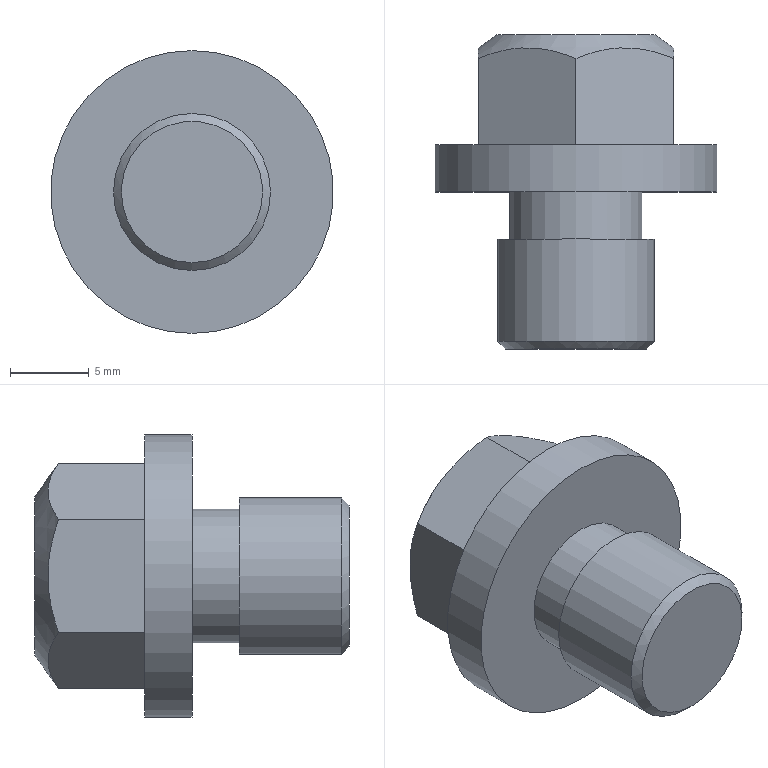Part | NX | 1 solid | 16 faces | box 18 x 20 x 18 mm | volume 2389 mm3 | plane 11 | cylinder 3 | cone 2 | commonest cylinder face diameters 8.5 x1 10 x1 18 x1
STEP:
#1=CARTESIAN_POINT('',(-6.227,18.49,-3.595));
#2=VERTEX_POINT('',#1);
#3=CARTESIAN_POINT('',(-6.227,18.49,3.595));
#4=VERTEX_POINT('',#3);
#5=CARTESIAN_POINT('',(-6.227,18.49,-3.595));
#6=CARTESIAN_POINT('',(-6.227,18.901,-2.433));
#7=CARTESIAN_POINT('',(-6.227,19.169,-1.246));
#8=CARTESIAN_POINT('',(-6.227,19.173,1.217));
#9=CARTESIAN_POINT('',(-6.227,18.902,2.429));
#10=CARTESIAN_POINT('',(-6.227,18.49,3.595));
#11=B_SPLINE_CURVE_WITH_KNOTS('',3,(#5,#6,#7,#8,#9,#10),.UNSPECIFIED.,.F.,.F.,(4,2,4),(0.,0.5,1.),.UNSPECIFIED.);
#12=EDGE_CURVE('',#2,#4,#11,.T.);
#13=ORIENTED_EDGE('',*,*,#12,.F.);
#14=CARTESIAN_POINT('',(-6.227,13.,-3.595));
#15=VERTEX_POINT('',#14);
#16=CARTESIAN_POINT('',(-6.227,20.,-3.595));
#17=DIRECTION('',(0.,-1.,0.));
#18=VECTOR('',#17,1.);
#19=LINE('',#16,#18);
#20=EDGE_CURVE('',#2,#15,#19,.T.);
#21=ORIENTED_EDGE('',*,*,#20,.T.);
#22=CARTESIAN_POINT('',(-6.227,13.,3.595));
#23=VERTEX_POINT('',#22);
#24=CARTESIAN_POINT('',(-6.227,13.,-3.595));
#25=DIRECTION('',(0.,0.,1.));
#26=VECTOR('',#25,1.);
#27=LINE('',#24,#26);
#28=EDGE_CURVE('',#15,#23,#27,.T.);
#29=ORIENTED_EDGE('',*,*,#28,.T.);
#30=CARTESIAN_POINT('',(-6.227,20.,3.595));
#31=DIRECTION('',(0.,-1.,0.));
#32=VECTOR('',#31,1.);
#33=LINE('',#30,#32);
#34=EDGE_CURVE('',#4,#23,#33,.T.);
#35=ORIENTED_EDGE('',*,*,#34,.F.);
#36=EDGE_LOOP('',(#13,#21,#29,#35));
#37=FACE_OUTER_BOUND('',#36,.T.);
#38=CARTESIAN_POINT('',(-6.227,20.,-3.595));
#39=DIRECTION('',(1.,0.,0.));
#40=DIRECTION('',(0.,0.,1.));
#41=AXIS2_PLACEMENT_3D('',#38,#39,#40);
#42=PLANE('',#41);
#43=ADVANCED_FACE('',(#37),#42,.F.);
#44=CARTESIAN_POINT('',(0.,18.49,7.19));
#45=VERTEX_POINT('',#44);
#46=CARTESIAN_POINT('',(-6.227,18.49,3.595));
#47=CARTESIAN_POINT('',(-5.22,18.901,4.176));
#48=CARTESIAN_POINT('',(-4.193,19.169,4.769));
#49=CARTESIAN_POINT('',(-2.059,19.173,6.001));
#50=CARTESIAN_POINT('',(-1.009,18.902,6.607));
#51=CARTESIAN_POINT('',(0.,18.49,7.19));
#52=B_SPLINE_CURVE_WITH_KNOTS('',3,(#46,#47,#48,#49,#50,#51),.UNSPECIFIED.,.F.,.F.,(4,2,4),(0.,0.5,1.),.UNSPECIFIED.);
#53=EDGE_CURVE('',#4,#45,#52,.T.);
#54=ORIENTED_EDGE('',*,*,#53,.F.);
#55=ORIENTED_EDGE('',*,*,#34,.T.);
#56=CARTESIAN_POINT('',(0.,13.,7.19));
#57=VERTEX_POINT('',#56);
#58=CARTESIAN_POINT('',(-6.227,13.,3.595));
#59=DIRECTION('',(0.866,0.,0.5));
#60=VECTOR('',#59,1.);
#61=LINE('',#58,#60);
#62=EDGE_CURVE('',#23,#57,#61,.T.);
#63=ORIENTED_EDGE('',*,*,#62,.T.);
#64=CARTESIAN_POINT('',(0.,20.,7.19));
#65=DIRECTION('',(0.,-1.,0.));
#66=VECTOR('',#65,1.);
#67=LINE('',#64,#66);
#68=EDGE_CURVE('',#45,#57,#67,.T.);
#69=ORIENTED_EDGE('',*,*,#68,.F.);
#70=EDGE_LOOP('',(#54,#55,#63,#69));
#71=FACE_OUTER_BOUND('',#70,.T.);
#72=CARTESIAN_POINT('',(-6.227,20.,3.595));
#73=DIRECTION('',(0.5,0.,-0.866));
#74=DIRECTION('',(0.866,0.,0.5));
#75=AXIS2_PLACEMENT_3D('',#72,#73,#74);
#76=PLANE('',#75);
#77=ADVANCED_FACE('',(#71),#76,.F.);
#78=CARTESIAN_POINT('',(6.227,18.49,3.595));
#79=VERTEX_POINT('',#78);
#80=CARTESIAN_POINT('',(0.,18.49,7.19));
#81=CARTESIAN_POINT('',(1.007,18.901,6.609));
#82=CARTESIAN_POINT('',(2.034,19.169,6.016));
#83=CARTESIAN_POINT('',(4.168,19.173,4.784));
#84=CARTESIAN_POINT('',(5.217,18.902,4.178));
#85=CARTESIAN_POINT('',(6.227,18.49,3.595));
#86=B_SPLINE_CURVE_WITH_KNOTS('',3,(#80,#81,#82,#83,#84,#85),.UNSPECIFIED.,.F.,.F.,(4,2,4),(0.,0.5,1.),.UNSPECIFIED.);
#87=EDGE_CURVE('',#45,#79,#86,.T.);
#88=ORIENTED_EDGE('',*,*,#87,.F.);
#89=ORIENTED_EDGE('',*,*,#68,.T.);
#90=CARTESIAN_POINT('',(6.227,13.,3.595));
#91=VERTEX_POINT('',#90);
#92=CARTESIAN_POINT('',(0.,13.,7.19));
#93=DIRECTION('',(0.866,0.,-0.5));
#94=VECTOR('',#93,1.);
#95=LINE('',#92,#94);
#96=EDGE_CURVE('',#57,#91,#95,.T.);
#97=ORIENTED_EDGE('',*,*,#96,.T.);
#98=CARTESIAN_POINT('',(6.227,20.,3.595));
#99=DIRECTION('',(0.,-1.,0.));
#100=VECTOR('',#99,1.);
#101=LINE('',#98,#100);
#102=EDGE_CURVE('',#79,#91,#101,.T.);
#103=ORIENTED_EDGE('',*,*,#102,.F.);
#104=EDGE_LOOP('',(#88,#89,#97,#103));
#105=FACE_OUTER_BOUND('',#104,.T.);
#106=CARTESIAN_POINT('',(0.,20.,7.19));
#107=DIRECTION('',(-0.5,0.,-0.866));
#108=DIRECTION('',(0.866,0.,-0.5));
#109=AXIS2_PLACEMENT_3D('',#106,#107,#108);
#110=PLANE('',#109);
#111=ADVANCED_FACE('',(#105),#110,.F.);
#112=CARTESIAN_POINT('',(6.227,18.49,-3.595));
#113=VERTEX_POINT('',#112);
#114=CARTESIAN_POINT('',(6.227,18.49,3.595));
#115=CARTESIAN_POINT('',(6.227,18.901,2.433));
#116=CARTESIAN_POINT('',(6.227,19.169,1.246));
#117=CARTESIAN_POINT('',(6.227,19.173,-1.217));
#118=CARTESIAN_POINT('',(6.227,18.902,-2.429));
#119=CARTESIAN_POINT('',(6.227,18.49,-3.595));
#120=B_SPLINE_CURVE_WITH_KNOTS('',3,(#114,#115,#116,#117,#118,#119),.UNSPECIFIED.,.F.,.F.,(4,2,4),(0.,0.5,1.),.UNSPECIFIED.);
#121=EDGE_CURVE('',#79,#113,#120,.T.);
#122=ORIENTED_EDGE('',*,*,#121,.F.);
#123=ORIENTED_EDGE('',*,*,#102,.T.);
#124=CARTESIAN_POINT('',(6.227,13.,-3.595));
#125=VERTEX_POINT('',#124);
#126=CARTESIAN_POINT('',(6.227,13.,3.595));
#127=DIRECTION('',(0.,0.,-1.));
#128=VECTOR('',#127,1.);
#129=LINE('',#126,#128);
#130=EDGE_CURVE('',#91,#125,#129,.T.);
#131=ORIENTED_EDGE('',*,*,#130,.T.);
#132=CARTESIAN_POINT('',(6.227,20.,-3.595));
#133=DIRECTION('',(0.,-1.,0.));
#134=VECTOR('',#133,1.);
#135=LINE('',#132,#134);
#136=EDGE_CURVE('',#113,#125,#135,.T.);
#137=ORIENTED_EDGE('',*,*,#136,.F.);
#138=EDGE_LOOP('',(#122,#123,#131,#137));
#139=FACE_OUTER_BOUND('',#138,.T.);
#140=CARTESIAN_POINT('',(6.227,20.,3.595));
#141=DIRECTION('',(-1.,0.,0.));
#142=DIRECTION('',(0.,0.,-1.));
#143=AXIS2_PLACEMENT_3D('',#140,#141,#142);
#144=PLANE('',#143);
#145=ADVANCED_FACE('',(#139),#144,.F.);
#146=CARTESIAN_POINT('',(0.,18.49,-7.19));
#147=VERTEX_POINT('',#146);
#148=CARTESIAN_POINT('',(6.227,18.49,-3.595));
#149=CARTESIAN_POINT('',(5.22,18.901,-4.176));
#150=CARTESIAN_POINT('',(4.193,19.169,-4.769));
#151=CARTESIAN_POINT('',(2.059,19.173,-6.001));
#152=CARTESIAN_POINT('',(1.009,18.902,-6.607));
#153=CARTESIAN_POINT('',(0.,18.49,-7.19));
#154=B_SPLINE_CURVE_WITH_KNOTS('',3,(#148,#149,#150,#151,#152,#153),.UNSPECIFIED.,.F.,.F.,(4,2,4),(0.,0.5,1.),.UNSPECIFIED.);
#155=EDGE_CURVE('',#113,#147,#154,.T.);
#156=ORIENTED_EDGE('',*,*,#155,.F.);
#157=ORIENTED_EDGE('',*,*,#136,.T.);
#158=CARTESIAN_POINT('',(0.,13.,-7.19));
#159=VERTEX_POINT('',#158);
#160=CARTESIAN_POINT('',(6.227,13.,-3.595));
#161=DIRECTION('',(-0.866,0.,-0.5));
#162=VECTOR('',#161,1.);
#163=LINE('',#160,#162);
#164=EDGE_CURVE('',#125,#159,#163,.T.);
#165=ORIENTED_EDGE('',*,*,#164,.T.);
#166=CARTESIAN_POINT('',(0.,20.,-7.19));
#167=DIRECTION('',(0.,-1.,0.));
#168=VECTOR('',#167,1.);
#169=LINE('',#166,#168);
#170=EDGE_CURVE('',#147,#159,#169,.T.);
#171=ORIENTED_EDGE('',*,*,#170,.F.);
#172=EDGE_LOOP('',(#156,#157,#165,#171));
#173=FACE_OUTER_BOUND('',#172,.T.);
#174=CARTESIAN_POINT('',(6.227,20.,-3.595));
#175=DIRECTION('',(-0.5,0.,0.866));
#176=DIRECTION('',(-0.866,0.,-0.5));
#177=AXIS2_PLACEMENT_3D('',#174,#175,#176);
#178=PLANE('',#177);
#179=ADVANCED_FACE('',(#173),#178,.F.);
#180=CARTESIAN_POINT('',(0.,18.49,-7.19));
#181=CARTESIAN_POINT('',(-1.007,18.901,-6.609));
#182=CARTESIAN_POINT('',(-2.034,19.169,-6.016));
#183=CARTESIAN_POINT('',(-4.168,19.173,-4.784));
#184=CARTESIAN_POINT('',(-5.217,18.902,-4.178));
#185=CARTESIAN_POINT('',(-6.227,18.49,-3.595));
#186=B_SPLINE_CURVE_WITH_KNOTS('',3,(#180,#181,#182,#183,#184,#185),.UNSPECIFIED.,.F.,.F.,(4,2,4),(0.,0.5,1.),.UNSPECIFIED.);
#187=EDGE_CURVE('',#147,#2,#186,.T.);
#188=ORIENTED_EDGE('',*,*,#187,.F.);
#189=ORIENTED_EDGE('',*,*,#170,.T.);
#190=CARTESIAN_POINT('',(0.,13.,-7.19));
#191=DIRECTION('',(-0.866,0.,0.5));
#192=VECTOR('',#191,1.);
#193=LINE('',#190,#192);
#194=EDGE_CURVE('',#159,#15,#193,.T.);
#195=ORIENTED_EDGE('',*,*,#194,.T.);
#196=ORIENTED_EDGE('',*,*,#20,.F.);
#197=EDGE_LOOP('',(#188,#189,#195,#196));
#198=FACE_OUTER_BOUND('',#197,.T.);
#199=CARTESIAN_POINT('',(0.,20.,-7.19));
#200=DIRECTION('',(0.5,0.,0.866));
#201=DIRECTION('',(-0.866,0.,0.5));
#202=AXIS2_PLACEMENT_3D('',#199,#200,#201);
#203=PLANE('',#202);
#204=ADVANCED_FACE('',(#198),#203,.F.);
#205=ORIENTED_EDGE('',*,*,#28,.F.);
#206=ORIENTED_EDGE('',*,*,#194,.F.);
#207=ORIENTED_EDGE('',*,*,#164,.F.);
#208=ORIENTED_EDGE('',*,*,#130,.F.);
#209=ORIENTED_EDGE('',*,*,#96,.F.);
#210=ORIENTED_EDGE('',*,*,#62,.F.);
#211=EDGE_LOOP('',(#205,#206,#207,#208,#209,#210));
#212=FACE_BOUND('',#211,.T.);
#213=CARTESIAN_POINT('',(0.,13.,-9.));
#214=VERTEX_POINT('',#213);
#215=CARTESIAN_POINT('',(0.,13.,0.));
#216=DIRECTION('',(0.,-1.,0.));
#217=DIRECTION('',(0.,0.,-1.));
#218=AXIS2_PLACEMENT_3D('',#215,#216,#217);
#219=CIRCLE('',#218,9.);
#220=EDGE_CURVE('',#214,#214,#219,.T.);
#221=ORIENTED_EDGE('',*,*,#220,.F.);
#222=EDGE_LOOP('',(#221));
#223=FACE_BOUND('',#222,.T.);
#224=CARTESIAN_POINT('',(9.,13.,0.));
#225=DIRECTION('',(0.,1.,0.));
#226=DIRECTION('',(0.,0.,-1.));
#227=AXIS2_PLACEMENT_3D('',#224,#225,#226);
#228=PLANE('',#227);
#229=ADVANCED_FACE('',(#212,#223),#228,.T.);
#230=ORIENTED_EDGE('',*,*,#220,.T.);
#231=EDGE_LOOP('',(#230));
#232=FACE_BOUND('',#231,.T.);
#233=CARTESIAN_POINT('',(0.,10.,-9.));
#234=VERTEX_POINT('',#233);
#235=CARTESIAN_POINT('',(0.,10.,0.));
#236=DIRECTION('',(0.,-1.,0.));
#237=DIRECTION('',(0.,0.,-1.));
#238=AXIS2_PLACEMENT_3D('',#235,#236,#237);
#239=CIRCLE('',#238,9.);
#240=EDGE_CURVE('',#234,#234,#239,.T.);
#241=ORIENTED_EDGE('',*,*,#240,.F.);
#242=EDGE_LOOP('',(#241));
#243=FACE_BOUND('',#242,.T.);
#244=CARTESIAN_POINT('',(0.,-7.,0.));
#245=DIRECTION('',(0.,-1.,0.));
#246=DIRECTION('',(0.,0.,1.));
#247=AXIS2_PLACEMENT_3D('',#244,#245,#246);
#248=CYLINDRICAL_SURFACE('',#247,9.);
#249=ADVANCED_FACE('',(#232,#243),#248,.T.);
#250=ORIENTED_EDGE('',*,*,#240,.T.);
#251=EDGE_LOOP('',(#250));
#252=FACE_BOUND('',#251,.T.);
#253=CARTESIAN_POINT('',(0.,10.,-4.25));
#254=VERTEX_POINT('',#253);
#255=CARTESIAN_POINT('',(0.,10.,0.));
#256=DIRECTION('',(0.,-1.,0.));
#257=DIRECTION('',(0.,0.,-1.));
#258=AXIS2_PLACEMENT_3D('',#255,#256,#257);
#259=CIRCLE('',#258,4.25);
#260=EDGE_CURVE('',#254,#254,#259,.T.);
#261=ORIENTED_EDGE('',*,*,#260,.F.);
#262=EDGE_LOOP('',(#261));
#263=FACE_BOUND('',#262,.T.);
#264=CARTESIAN_POINT('',(4.25,10.,0.));
#265=DIRECTION('',(0.,-1.,0.));
#266=DIRECTION('',(0.,0.,1.));
#267=AXIS2_PLACEMENT_3D('',#264,#265,#266);
#268=PLANE('',#267);
#269=ADVANCED_FACE('',(#252,#263),#268,.T.);
#270=ORIENTED_EDGE('',*,*,#260,.T.);
#271=EDGE_LOOP('',(#270));
#272=FACE_BOUND('',#271,.T.);
#273=CARTESIAN_POINT('',(0.,7.,-4.25));
#274=VERTEX_POINT('',#273);
#275=CARTESIAN_POINT('',(0.,7.,0.));
#276=DIRECTION('',(0.,-1.,0.));
#277=DIRECTION('',(0.,0.,-1.));
#278=AXIS2_PLACEMENT_3D('',#275,#276,#277);
#279=CIRCLE('',#278,4.25);
#280=EDGE_CURVE('',#274,#274,#279,.T.);
#281=ORIENTED_EDGE('',*,*,#280,.F.);
#282=EDGE_LOOP('',(#281));
#283=FACE_BOUND('',#282,.T.);
#284=CARTESIAN_POINT('',(0.,-7.,0.));
#285=DIRECTION('',(0.,-1.,0.));
#286=DIRECTION('',(0.,0.,1.));
#287=AXIS2_PLACEMENT_3D('',#284,#285,#286);
#288=CYLINDRICAL_SURFACE('',#287,4.25);
#289=ADVANCED_FACE('',(#272,#283),#288,.T.);
#290=ORIENTED_EDGE('',*,*,#280,.T.);
#291=EDGE_LOOP('',(#290));
#292=FACE_BOUND('',#291,.T.);
#293=CARTESIAN_POINT('',(0.,7.,-5.));
#294=VERTEX_POINT('',#293);
#295=CARTESIAN_POINT('',(0.,7.,0.));
#296=DIRECTION('',(0.,-1.,0.));
#297=DIRECTION('',(0.,0.,-1.));
#298=AXIS2_PLACEMENT_3D('',#295,#296,#297);
#299=CIRCLE('',#298,5.);
#300=EDGE_CURVE('',#294,#294,#299,.T.);
#301=ORIENTED_EDGE('',*,*,#300,.F.);
#302=EDGE_LOOP('',(#301));
#303=FACE_BOUND('',#302,.T.);
#304=CARTESIAN_POINT('',(5.,7.,0.));
#305=DIRECTION('',(0.,1.,0.));
#306=DIRECTION('',(0.,0.,-1.));
#307=AXIS2_PLACEMENT_3D('',#304,#305,#306);
#308=PLANE('',#307);
#309=ADVANCED_FACE('',(#292,#303),#308,.T.);
#310=ORIENTED_EDGE('',*,*,#300,.T.);
#311=EDGE_LOOP('',(#310));
#312=FACE_BOUND('',#311,.T.);
#313=CARTESIAN_POINT('',(0.,0.5,-5.));
#314=VERTEX_POINT('',#313);
#315=CARTESIAN_POINT('',(0.,0.5,0.));
#316=DIRECTION('',(0.,-1.,0.));
#317=DIRECTION('',(0.,0.,-1.));
#318=AXIS2_PLACEMENT_3D('',#315,#316,#317);
#319=CIRCLE('',#318,5.);
#320=EDGE_CURVE('',#314,#314,#319,.T.);
#321=ORIENTED_EDGE('',*,*,#320,.F.);
#322=EDGE_LOOP('',(#321));
#323=FACE_BOUND('',#322,.T.);
#324=CARTESIAN_POINT('',(0.,-7.,0.));
#325=DIRECTION('',(0.,-1.,0.));
#326=DIRECTION('',(0.,0.,1.));
#327=AXIS2_PLACEMENT_3D('',#324,#325,#326);
#328=CYLINDRICAL_SURFACE('',#327,5.);
#329=ADVANCED_FACE('',(#312,#323),#328,.T.);
#330=ORIENTED_EDGE('',*,*,#320,.T.);
#331=EDGE_LOOP('',(#330));
#332=FACE_BOUND('',#331,.T.);
#333=CARTESIAN_POINT('',(0.,0.,-4.5));
#334=VERTEX_POINT('',#333);
#335=CARTESIAN_POINT('',(0.,0.,0.));
#336=DIRECTION('',(0.,-1.,0.));
#337=DIRECTION('',(0.,0.,-1.));
#338=AXIS2_PLACEMENT_3D('',#335,#336,#337);
#339=CIRCLE('',#338,4.5);
#340=EDGE_CURVE('',#334,#334,#339,.T.);
#341=ORIENTED_EDGE('',*,*,#340,.F.);
#342=EDGE_LOOP('',(#341));
#343=FACE_BOUND('',#342,.T.);
#344=CARTESIAN_POINT('',(0.,0.,0.));
#345=DIRECTION('',(0.,1.,0.));
#346=DIRECTION('',(0.,0.,-1.));
#347=AXIS2_PLACEMENT_3D('',#344,#345,#346);
#348=CONICAL_SURFACE('',#347,4.5,45.);
#349=ADVANCED_FACE('',(#332,#343),#348,.T.);
#350=ORIENTED_EDGE('',*,*,#340,.T.);
#351=EDGE_LOOP('',(#350));
#352=FACE_OUTER_BOUND('',#351,.T.);
#353=CARTESIAN_POINT('',(0.,0.,0.));
#354=DIRECTION('',(0.,-1.,0.));
#355=DIRECTION('',(0.,0.,1.));
#356=AXIS2_PLACEMENT_3D('',#353,#354,#355);
#357=PLANE('',#356);
#358=ADVANCED_FACE('',(#352),#357,.T.);
#359=CARTESIAN_POINT('',(0.,20.,5.054));
#360=VERTEX_POINT('',#359);
#361=CARTESIAN_POINT('',(0.,20.,0.));
#362=DIRECTION('',(0.,1.,0.));
#363=DIRECTION('',(0.,0.,1.));
#364=AXIS2_PLACEMENT_3D('',#361,#362,#363);
#365=CIRCLE('',#364,5.054);
#366=EDGE_CURVE('',#360,#360,#365,.T.);
#367=ORIENTED_EDGE('',*,*,#366,.F.);
#368=EDGE_LOOP('',(#367));
#369=FACE_BOUND('',#368,.T.);
#370=ORIENTED_EDGE('',*,*,#187,.T.);
#371=ORIENTED_EDGE('',*,*,#12,.T.);
#372=ORIENTED_EDGE('',*,*,#53,.T.);
#373=ORIENTED_EDGE('',*,*,#87,.T.);
#374=ORIENTED_EDGE('',*,*,#121,.T.);
#375=ORIENTED_EDGE('',*,*,#155,.T.);
#376=EDGE_LOOP('',(#370,#371,#372,#373,#374,#375));
#377=FACE_BOUND('',#376,.T.);
#378=CARTESIAN_POINT('',(0.,19.839,0.));
#379=DIRECTION('',(0.,-1.,0.));
#380=DIRECTION('',(0.,0.,1.));
#381=AXIS2_PLACEMENT_3D('',#378,#379,#380);
#382=CONICAL_SURFACE('',#381,5.282,54.74);
#383=ADVANCED_FACE('',(#369,#377),#382,.T.);
#384=ORIENTED_EDGE('',*,*,#366,.T.);
#385=EDGE_LOOP('',(#384));
#386=FACE_OUTER_BOUND('',#385,.T.);
#387=CARTESIAN_POINT('',(0.,20.,0.));
#388=DIRECTION('',(0.,1.,0.));
#389=DIRECTION('',(0.,0.,-1.));
#390=AXIS2_PLACEMENT_3D('',#387,#388,#389);
#391=PLANE('',#390);
#392=ADVANCED_FACE('',(#386),#391,.T.);
#393=CLOSED_SHELL('',(#43,#77,#111,#145,#179,#204,#229,#249,#269,#289,#309,#329,#349,#358,#383,#392));
#394=MANIFOLD_SOLID_BREP('',#393);
#395=(LENGTH_UNIT()NAMED_UNIT(*)SI_UNIT(.MILLI.,.METRE.));
#396=UNCERTAINTY_MEASURE_WITH_UNIT(LENGTH_MEASURE(0.0508),#395,'','');
#397=(NAMED_UNIT(*)PLANE_ANGLE_UNIT()SI_UNIT($,.RADIAN.));
#398=PLANE_ANGLE_MEASURE_WITH_UNIT(PLANE_ANGLE_MEASURE(0.01745),#397);
#399=DIMENSIONAL_EXPONENTS(0.,0.,0.,0.,0.,0.,0.);
#400=(CONVERSION_BASED_UNIT('DEGREE',#398)NAMED_UNIT(#399)PLANE_ANGLE_UNIT());
#401=(NAMED_UNIT(*)SI_UNIT($,.STERADIAN.)SOLID_ANGLE_UNIT());
#402=(GEOMETRIC_REPRESENTATION_CONTEXT(3)GLOBAL_UNCERTAINTY_ASSIGNED_CONTEXT((#396))GLOBAL_UNIT_ASSIGNED_CONTEXT((#395,#400,#401))REPRESENTATION_CONTEXT('',''));
#403=ADVANCED_BREP_SHAPE_REPRESENTATION('',(#394),#402);